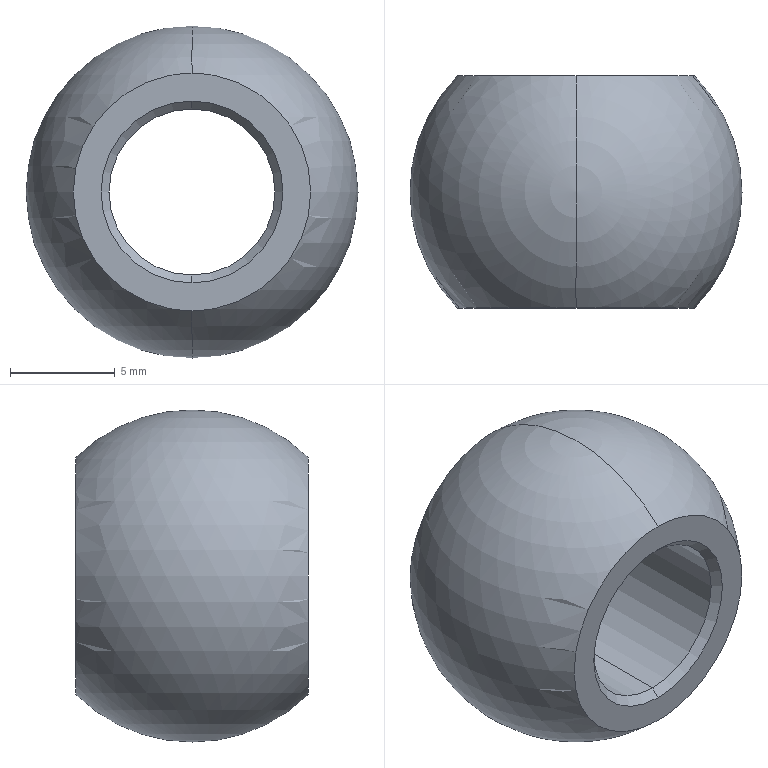Part | NX | features LUMP2 2 | 1 solid | 10 faces | box 15.875 x 11.1 x 15.875 mm | volume 1286 mm3 | cone 4 | cylinder 2 | plane 2 | sphere 2 | commonest cylinder face diameters 7.938 x2
STEP:
#1=CARTESIAN_POINT('',(0.,5.169,30.956));
#2=VERTEX_POINT('',#1);
#3=CARTESIAN_POINT('',(0.,-5.169,30.956));
#4=VERTEX_POINT('',#3);
#5=CARTESIAN_POINT('',(0.,0.,30.956));
#6=DIRECTION('',(0.,-1.,0.));
#7=VECTOR('',#6,1000.);
#8=LINE('',#5,#7);
#9=EDGE_CURVE('',#2,#4,#8,.T.);
#10=ORIENTED_EDGE('',*,*,#9,.F.);
#11=CARTESIAN_POINT('',(0.,5.169,38.894));
#12=VERTEX_POINT('',#11);
#13=CARTESIAN_POINT('',(0.,5.169,34.925));
#14=DIRECTION('',(0.,1.,0.));
#15=DIRECTION('',(0.,0.,-1.));
#16=AXIS2_PLACEMENT_3D('',#13,#14,#15);
#17=CIRCLE('',#16,3.969);
#18=EDGE_CURVE('',#2,#12,#17,.T.);
#19=ORIENTED_EDGE('',*,*,#18,.T.);
#20=CARTESIAN_POINT('',(0.,-5.169,38.894));
#21=VERTEX_POINT('',#20);
#22=CARTESIAN_POINT('',(0.,0.,38.894));
#23=DIRECTION('',(0.,1.,0.));
#24=VECTOR('',#23,1000.);
#25=LINE('',#22,#24);
#26=EDGE_CURVE('',#21,#12,#25,.T.);
#27=ORIENTED_EDGE('',*,*,#26,.F.);
#28=CARTESIAN_POINT('',(0.,-5.169,34.925));
#29=DIRECTION('',(0.,-1.,0.));
#30=DIRECTION('',(0.,0.,-1.));
#31=AXIS2_PLACEMENT_3D('',#28,#29,#30);
#32=CIRCLE('',#31,3.969);
#33=EDGE_CURVE('',#21,#4,#32,.T.);
#34=ORIENTED_EDGE('',*,*,#33,.T.);
#35=EDGE_LOOP('',(#10,#19,#27,#34));
#36=FACE_BOUND('',#35,.T.);
#37=CARTESIAN_POINT('',(0.,0.,34.925));
#38=DIRECTION('',(0.,1.,0.));
#39=DIRECTION('',(0.,0.,1.));
#40=AXIS2_PLACEMENT_3D('',#37,#38,#39);
#41=CYLINDRICAL_SURFACE('',#40,3.969);
#42=ADVANCED_FACE('',(#36),#41,.F.);
#43=ORIENTED_EDGE('',*,*,#9,.T.);
#44=CARTESIAN_POINT('',(0.,-5.169,34.925));
#45=DIRECTION('',(0.,-1.,0.));
#46=DIRECTION('',(0.,0.,-1.));
#47=AXIS2_PLACEMENT_3D('',#44,#45,#46);
#48=CIRCLE('',#47,3.969);
#49=EDGE_CURVE('',#4,#21,#48,.T.);
#50=ORIENTED_EDGE('',*,*,#49,.T.);
#51=ORIENTED_EDGE('',*,*,#26,.T.);
#52=CARTESIAN_POINT('',(0.,5.169,34.925));
#53=DIRECTION('',(0.,1.,0.));
#54=DIRECTION('',(0.,0.,-1.));
#55=AXIS2_PLACEMENT_3D('',#52,#53,#54);
#56=CIRCLE('',#55,3.969);
#57=EDGE_CURVE('',#12,#2,#56,.T.);
#58=ORIENTED_EDGE('',*,*,#57,.T.);
#59=EDGE_LOOP('',(#43,#50,#51,#58));
#60=FACE_BOUND('',#59,.T.);
#61=CARTESIAN_POINT('',(0.,0.,34.925));
#62=DIRECTION('',(0.,1.,0.));
#63=DIRECTION('',(0.,0.,1.));
#64=AXIS2_PLACEMENT_3D('',#61,#62,#63);
#65=CYLINDRICAL_SURFACE('',#64,3.969);
#66=ADVANCED_FACE('',(#60),#65,.F.);
#67=CARTESIAN_POINT('',(0.,-5.55,30.575));
#68=VERTEX_POINT('',#67);
#69=CARTESIAN_POINT('',(0.,-5.359,30.766));
#70=DIRECTION('',(0.,-0.7071,-0.7071));
#71=VECTOR('',#70,1000.);
#72=LINE('',#69,#71);
#73=EDGE_CURVE('',#4,#68,#72,.T.);
#74=ORIENTED_EDGE('',*,*,#73,.T.);
#75=CARTESIAN_POINT('',(0.,-5.55,39.275));
#76=VERTEX_POINT('',#75);
#77=CARTESIAN_POINT('',(0.,-5.55,34.925));
#78=DIRECTION('',(0.,1.,0.));
#79=DIRECTION('',(0.,0.,-1.));
#80=AXIS2_PLACEMENT_3D('',#77,#78,#79);
#81=CIRCLE('',#80,4.35);
#82=EDGE_CURVE('',#76,#68,#81,.T.);
#83=ORIENTED_EDGE('',*,*,#82,.F.);
#84=CARTESIAN_POINT('',(0.,-5.359,39.084));
#85=DIRECTION('',(0.,0.7071,-0.7071));
#86=VECTOR('',#85,1000.);
#87=LINE('',#84,#86);
#88=EDGE_CURVE('',#76,#21,#87,.T.);
#89=ORIENTED_EDGE('',*,*,#88,.T.);
#90=ORIENTED_EDGE('',*,*,#49,.F.);
#91=EDGE_LOOP('',(#74,#83,#89,#90));
#92=FACE_BOUND('',#91,.T.);
#93=CARTESIAN_POINT('',(0.,-5.359,34.925));
#94=DIRECTION('',(0.,-1.,0.));
#95=DIRECTION('',(0.,0.,1.));
#96=AXIS2_PLACEMENT_3D('',#93,#94,#95);
#97=CONICAL_SURFACE('',#96,4.159,0.7854);
#98=ADVANCED_FACE('',(#92),#97,.F.);
#99=ORIENTED_EDGE('',*,*,#73,.F.);
#100=ORIENTED_EDGE('',*,*,#33,.F.);
#101=ORIENTED_EDGE('',*,*,#88,.F.);
#102=CARTESIAN_POINT('',(0.,-5.55,34.925));
#103=DIRECTION('',(0.,1.,0.));
#104=DIRECTION('',(0.,0.,-1.));
#105=AXIS2_PLACEMENT_3D('',#102,#103,#104);
#106=CIRCLE('',#105,4.35);
#107=EDGE_CURVE('',#68,#76,#106,.T.);
#108=ORIENTED_EDGE('',*,*,#107,.F.);
#109=EDGE_LOOP('',(#99,#100,#101,#108));
#110=FACE_BOUND('',#109,.T.);
#111=CARTESIAN_POINT('',(0.,-5.359,34.925));
#112=DIRECTION('',(0.,-1.,0.));
#113=DIRECTION('',(0.,0.,1.));
#114=AXIS2_PLACEMENT_3D('',#111,#112,#113);
#115=CONICAL_SURFACE('',#114,4.159,0.7854);
#116=ADVANCED_FACE('',(#110),#115,.F.);
#117=CARTESIAN_POINT('',(0.,5.55,30.575));
#118=VERTEX_POINT('',#117);
#119=CARTESIAN_POINT('',(0.,5.359,30.766));
#120=DIRECTION('',(0.,0.7071,-0.7071));
#121=VECTOR('',#120,1000.);
#122=LINE('',#119,#121);
#123=EDGE_CURVE('',#2,#118,#122,.T.);
#124=ORIENTED_EDGE('',*,*,#123,.T.);
#125=CARTESIAN_POINT('',(0.,5.55,39.275));
#126=VERTEX_POINT('',#125);
#127=CARTESIAN_POINT('',(0.,5.55,34.925));
#128=DIRECTION('',(0.,-1.,0.));
#129=DIRECTION('',(0.,0.,-1.));
#130=AXIS2_PLACEMENT_3D('',#127,#128,#129);
#131=CIRCLE('',#130,4.35);
#132=EDGE_CURVE('',#126,#118,#131,.T.);
#133=ORIENTED_EDGE('',*,*,#132,.F.);
#134=CARTESIAN_POINT('',(0.,5.359,39.084));
#135=DIRECTION('',(0.,-0.7071,-0.7071));
#136=VECTOR('',#135,1000.);
#137=LINE('',#134,#136);
#138=EDGE_CURVE('',#126,#12,#137,.T.);
#139=ORIENTED_EDGE('',*,*,#138,.T.);
#140=ORIENTED_EDGE('',*,*,#18,.F.);
#141=EDGE_LOOP('',(#124,#133,#139,#140));
#142=FACE_BOUND('',#141,.T.);
#143=CARTESIAN_POINT('',(0.,5.359,34.925));
#144=DIRECTION('',(0.,1.,0.));
#145=DIRECTION('',(0.,0.,1.));
#146=AXIS2_PLACEMENT_3D('',#143,#144,#145);
#147=CONICAL_SURFACE('',#146,4.159,0.7854);
#148=ADVANCED_FACE('',(#142),#147,.F.);
#149=ORIENTED_EDGE('',*,*,#123,.F.);
#150=ORIENTED_EDGE('',*,*,#57,.F.);
#151=ORIENTED_EDGE('',*,*,#138,.F.);
#152=CARTESIAN_POINT('',(0.,5.55,34.925));
#153=DIRECTION('',(0.,-1.,0.));
#154=DIRECTION('',(0.,0.,-1.));
#155=AXIS2_PLACEMENT_3D('',#152,#153,#154);
#156=CIRCLE('',#155,4.35);
#157=EDGE_CURVE('',#118,#126,#156,.T.);
#158=ORIENTED_EDGE('',*,*,#157,.F.);
#159=EDGE_LOOP('',(#149,#150,#151,#158));
#160=FACE_BOUND('',#159,.T.);
#161=CARTESIAN_POINT('',(0.,5.359,34.925));
#162=DIRECTION('',(0.,1.,0.));
#163=DIRECTION('',(0.,0.,1.));
#164=AXIS2_PLACEMENT_3D('',#161,#162,#163);
#165=CONICAL_SURFACE('',#164,4.159,0.7854);
#166=ADVANCED_FACE('',(#160),#165,.F.);
#167=ORIENTED_EDGE('',*,*,#107,.T.);
#168=ORIENTED_EDGE('',*,*,#82,.T.);
#169=EDGE_LOOP('',(#167,#168));
#170=FACE_BOUND('',#169,.T.);
#171=CARTESIAN_POINT('',(0.,-5.55,40.6));
#172=VERTEX_POINT('',#171);
#173=CARTESIAN_POINT('',(0.,-5.55,29.25));
#174=VERTEX_POINT('',#173);
#175=CARTESIAN_POINT('',(0.,-5.55,34.925));
#176=DIRECTION('',(0.,1.,0.));
#177=DIRECTION('',(0.,0.,-1.));
#178=AXIS2_PLACEMENT_3D('',#175,#176,#177);
#179=CIRCLE('',#178,5.675);
#180=EDGE_CURVE('',#172,#174,#179,.T.);
#181=ORIENTED_EDGE('',*,*,#180,.F.);
#182=CARTESIAN_POINT('',(0.,-5.55,34.925));
#183=DIRECTION('',(0.,1.,0.));
#184=DIRECTION('',(0.,0.,-1.));
#185=AXIS2_PLACEMENT_3D('',#182,#183,#184);
#186=CIRCLE('',#185,5.675);
#187=EDGE_CURVE('',#174,#172,#186,.T.);
#188=ORIENTED_EDGE('',*,*,#187,.F.);
#189=EDGE_LOOP('',(#181,#188));
#190=FACE_BOUND('',#189,.T.);
#191=CARTESIAN_POINT('',(0.,-5.55,34.925));
#192=DIRECTION('',(0.,1.,0.));
#193=DIRECTION('',(-1.,0.,0.));
#194=AXIS2_PLACEMENT_3D('',#191,#192,#193);
#195=PLANE('',#194);
#196=ADVANCED_FACE('',(#170,#190),#195,.F.);
#197=ORIENTED_EDGE('',*,*,#157,.T.);
#198=ORIENTED_EDGE('',*,*,#132,.T.);
#199=EDGE_LOOP('',(#197,#198));
#200=FACE_BOUND('',#199,.T.);
#201=CARTESIAN_POINT('',(0.,5.55,29.25));
#202=VERTEX_POINT('',#201);
#203=CARTESIAN_POINT('',(0.,5.55,40.6));
#204=VERTEX_POINT('',#203);
#205=CARTESIAN_POINT('',(0.,5.55,34.925));
#206=DIRECTION('',(0.,-1.,0.));
#207=DIRECTION('',(0.,0.,1.));
#208=AXIS2_PLACEMENT_3D('',#205,#206,#207);
#209=CIRCLE('',#208,5.675);
#210=EDGE_CURVE('',#202,#204,#209,.T.);
#211=ORIENTED_EDGE('',*,*,#210,.F.);
#212=CARTESIAN_POINT('',(0.,5.55,34.925));
#213=DIRECTION('',(0.,-1.,0.));
#214=DIRECTION('',(0.,0.,1.));
#215=AXIS2_PLACEMENT_3D('',#212,#213,#214);
#216=CIRCLE('',#215,5.675);
#217=EDGE_CURVE('',#204,#202,#216,.T.);
#218=ORIENTED_EDGE('',*,*,#217,.F.);
#219=EDGE_LOOP('',(#211,#218));
#220=FACE_BOUND('',#219,.T.);
#221=CARTESIAN_POINT('',(0.,5.55,34.925));
#222=DIRECTION('',(0.,-1.,0.));
#223=DIRECTION('',(-1.,0.,0.));
#224=AXIS2_PLACEMENT_3D('',#221,#222,#223);
#225=PLANE('',#224);
#226=ADVANCED_FACE('',(#200,#220),#225,.F.);
#227=CARTESIAN_POINT('',(0.,0.,26.988));
#228=VERTEX_POINT('',#227);
#229=CARTESIAN_POINT('',(0.,0.,34.925));
#230=DIRECTION('',(1.,0.,0.));
#231=DIRECTION('',(0.,0.,1.));
#232=AXIS2_PLACEMENT_3D('',#229,#230,#231);
#233=CIRCLE('',#232,7.938);
#234=EDGE_CURVE('',#174,#228,#233,.T.);
#235=ORIENTED_EDGE('',*,*,#234,.F.);
#236=ORIENTED_EDGE('',*,*,#187,.T.);
#237=CARTESIAN_POINT('',(0.,0.,42.862));
#238=VERTEX_POINT('',#237);
#239=CARTESIAN_POINT('',(0.,0.,34.925));
#240=DIRECTION('',(1.,0.,0.));
#241=DIRECTION('',(0.,0.,1.));
#242=AXIS2_PLACEMENT_3D('',#239,#240,#241);
#243=CIRCLE('',#242,7.938);
#244=EDGE_CURVE('',#238,#172,#243,.T.);
#245=ORIENTED_EDGE('',*,*,#244,.F.);
#246=CARTESIAN_POINT('',(0.,0.,34.925));
#247=DIRECTION('',(1.,0.,0.));
#248=DIRECTION('',(0.,0.,1.));
#249=AXIS2_PLACEMENT_3D('',#246,#247,#248);
#250=CIRCLE('',#249,7.938);
#251=EDGE_CURVE('',#204,#238,#250,.T.);
#252=ORIENTED_EDGE('',*,*,#251,.F.);
#253=ORIENTED_EDGE('',*,*,#217,.T.);
#254=CARTESIAN_POINT('',(0.,0.,34.925));
#255=DIRECTION('',(1.,0.,0.));
#256=DIRECTION('',(0.,0.,1.));
#257=AXIS2_PLACEMENT_3D('',#254,#255,#256);
#258=CIRCLE('',#257,7.938);
#259=EDGE_CURVE('',#228,#202,#258,.T.);
#260=ORIENTED_EDGE('',*,*,#259,.F.);
#261=EDGE_LOOP('',(#235,#236,#245,#252,#253,#260));
#262=FACE_BOUND('',#261,.T.);
#263=CARTESIAN_POINT('',(0.,0.,34.925));
#264=DIRECTION('',(0.,0.,1.));
#265=DIRECTION('',(-1.,0.,0.));
#266=AXIS2_PLACEMENT_3D('',#263,#264,#265);
#267=SPHERICAL_SURFACE('',#266,7.938);
#268=ADVANCED_FACE('',(#262),#267,.T.);
#269=ORIENTED_EDGE('',*,*,#234,.T.);
#270=ORIENTED_EDGE('',*,*,#259,.T.);
#271=ORIENTED_EDGE('',*,*,#210,.T.);
#272=ORIENTED_EDGE('',*,*,#251,.T.);
#273=ORIENTED_EDGE('',*,*,#244,.T.);
#274=ORIENTED_EDGE('',*,*,#180,.T.);
#275=EDGE_LOOP('',(#269,#270,#271,#272,#273,#274));
#276=FACE_BOUND('',#275,.T.);
#277=CARTESIAN_POINT('',(0.,0.,34.925));
#278=DIRECTION('',(0.,0.,1.));
#279=DIRECTION('',(-1.,0.,0.));
#280=AXIS2_PLACEMENT_3D('',#277,#278,#279);
#281=SPHERICAL_SURFACE('',#280,7.938);
#282=ADVANCED_FACE('',(#276),#281,.T.);
#283=CLOSED_SHELL('',(#42,#66,#98,#116,#148,#166,#196,#226,#268,#282));
#284=MANIFOLD_SOLID_BREP('',#283);
#285=(LENGTH_UNIT()NAMED_UNIT(*)SI_UNIT(.MILLI.,.METRE.));
#286=UNCERTAINTY_MEASURE_WITH_UNIT(LENGTH_MEASURE(0.00001),#285,'','');
#287=(NAMED_UNIT(*)PLANE_ANGLE_UNIT()SI_UNIT($,.RADIAN.));
#288=(NAMED_UNIT(*)SI_UNIT($,.STERADIAN.)SOLID_ANGLE_UNIT());
#289=(GEOMETRIC_REPRESENTATION_CONTEXT(3)GLOBAL_UNCERTAINTY_ASSIGNED_CONTEXT((#286))GLOBAL_UNIT_ASSIGNED_CONTEXT((#285,#287,#288))REPRESENTATION_CONTEXT('',''));
#290=ADVANCED_BREP_SHAPE_REPRESENTATION('',(#284),#289);